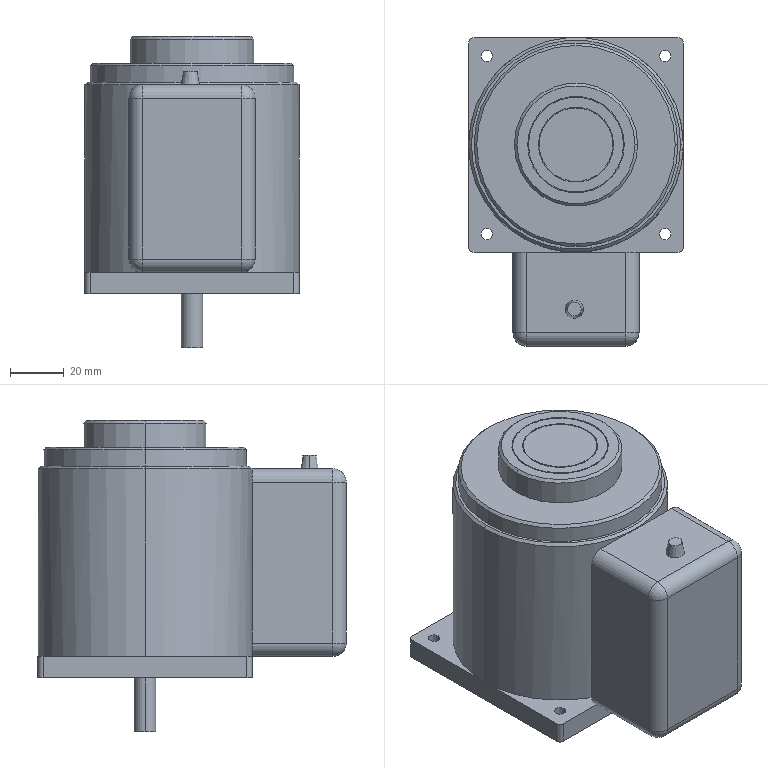Part | SolidWorks | features ICE 7, Fillet 2, 3DProfileFeature 1, Chamfer 1, Extrusion 1, HoleWzd 1 | 2 solids | 72 faces | box 80 x 115 x 116 mm | volume 570040 mm3 | cylinder 36 | plane 24 | cone 8 | sphere 4 | commonest cylinder face diameters 4.2 x8 10 x8 4 x4 8 x2 27.5 x2 28 x2